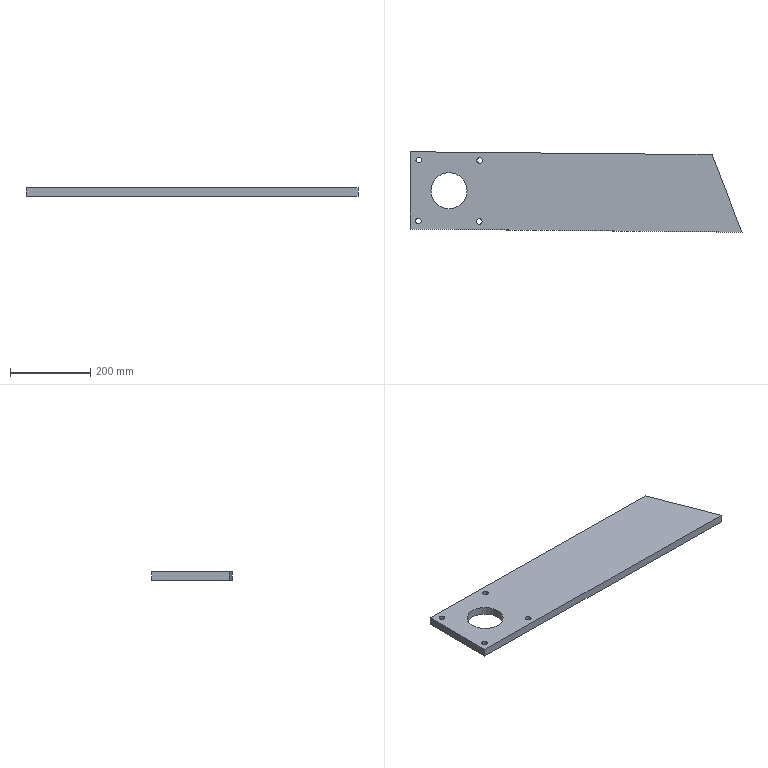Part | SolidWorks | features BaseBody 1 | 1 solid | 16 faces | box 828.827 x 200.894 x 20 mm | volume 2911165 mm3 | cylinder 10 | plane 6 | commonest cylinder face diameters 14.376 x6 14.371 x2 90 x2
STEP:
#1=CARTESIAN_POINT('',(1275.714,2622.106,20.));
#2=VERTEX_POINT('',#1);
#3=CARTESIAN_POINT('',(1290.09,2622.106,20.));
#4=VERTEX_POINT('',#3);
#5=CARTESIAN_POINT('',(1282.902,2622.106,20.));
#6=DIRECTION('',(0.,0.,1.));
#7=DIRECTION('',(1.,0.,0.));
#8=AXIS2_PLACEMENT_3D('',#5,#6,#7);
#9=CIRCLE('',#8,7.188);
#10=EDGE_CURVE('',#2,#4,#9,.T.);
#11=ORIENTED_EDGE('',*,*,#10,.T.);
#12=CARTESIAN_POINT('',(1290.09,2622.106,0.));
#13=VERTEX_POINT('',#12);
#14=CARTESIAN_POINT('',(1290.09,2622.106,20.));
#15=DIRECTION('',(0.,0.,-1.));
#16=VECTOR('',#15,1000.);
#17=LINE('',#14,#16);
#18=EDGE_CURVE('',#4,#13,#17,.T.);
#19=ORIENTED_EDGE('',*,*,#18,.T.);
#20=CARTESIAN_POINT('',(1275.714,2622.106,0.));
#21=VERTEX_POINT('',#20);
#22=CARTESIAN_POINT('',(1282.902,2622.106,0.));
#23=DIRECTION('',(0.,0.,1.));
#24=DIRECTION('',(1.,0.,0.));
#25=AXIS2_PLACEMENT_3D('',#22,#23,#24);
#26=CIRCLE('',#25,7.188);
#27=EDGE_CURVE('',#21,#13,#26,.T.);
#28=ORIENTED_EDGE('',*,*,#27,.F.);
#29=CARTESIAN_POINT('',(1275.714,2622.106,20.));
#30=DIRECTION('',(0.,0.,-1.));
#31=VECTOR('',#30,1000.);
#32=LINE('',#29,#31);
#33=EDGE_CURVE('',#2,#21,#32,.T.);
#34=ORIENTED_EDGE('',*,*,#33,.F.);
#35=EDGE_LOOP('',(#11,#19,#28,#34));
#36=FACE_OUTER_BOUND('',#35,.T.);
#37=CARTESIAN_POINT('',(1282.902,2622.106,20.));
#38=DIRECTION('',(0.,0.,-1.));
#39=DIRECTION('',(-1.,0.,0.));
#40=AXIS2_PLACEMENT_3D('',#37,#38,#39);
#41=CYLINDRICAL_SURFACE('',#40,7.188);
#42=ADVANCED_FACE('',(#36),#41,.F.);
#43=CARTESIAN_POINT('',(1427.707,2620.657,20.));
#44=VERTEX_POINT('',#43);
#45=CARTESIAN_POINT('',(1442.083,2620.657,20.));
#46=VERTEX_POINT('',#45);
#47=CARTESIAN_POINT('',(1434.895,2620.657,20.));
#48=DIRECTION('',(0.,0.,1.));
#49=DIRECTION('',(1.,0.,0.));
#50=AXIS2_PLACEMENT_3D('',#47,#48,#49);
#51=CIRCLE('',#50,7.188);
#52=EDGE_CURVE('',#44,#46,#51,.T.);
#53=ORIENTED_EDGE('',*,*,#52,.T.);
#54=CARTESIAN_POINT('',(1442.083,2620.657,0.));
#55=VERTEX_POINT('',#54);
#56=CARTESIAN_POINT('',(1442.083,2620.657,20.));
#57=DIRECTION('',(0.,0.,-1.));
#58=VECTOR('',#57,1000.);
#59=LINE('',#56,#58);
#60=EDGE_CURVE('',#46,#55,#59,.T.);
#61=ORIENTED_EDGE('',*,*,#60,.T.);
#62=CARTESIAN_POINT('',(1427.707,2620.657,0.));
#63=VERTEX_POINT('',#62);
#64=CARTESIAN_POINT('',(1434.895,2620.657,0.));
#65=DIRECTION('',(0.,0.,1.));
#66=DIRECTION('',(1.,0.,0.));
#67=AXIS2_PLACEMENT_3D('',#64,#65,#66);
#68=CIRCLE('',#67,7.188);
#69=EDGE_CURVE('',#63,#55,#68,.T.);
#70=ORIENTED_EDGE('',*,*,#69,.F.);
#71=CARTESIAN_POINT('',(1427.707,2620.657,20.));
#72=DIRECTION('',(0.,0.,-1.));
#73=VECTOR('',#72,1000.);
#74=LINE('',#71,#73);
#75=EDGE_CURVE('',#44,#63,#74,.T.);
#76=ORIENTED_EDGE('',*,*,#75,.F.);
#77=EDGE_LOOP('',(#53,#61,#70,#76));
#78=FACE_OUTER_BOUND('',#77,.T.);
#79=CARTESIAN_POINT('',(1434.895,2620.657,20.));
#80=DIRECTION('',(0.,0.,-1.));
#81=DIRECTION('',(-1.,0.,0.));
#82=AXIS2_PLACEMENT_3D('',#79,#80,#81);
#83=CYLINDRICAL_SURFACE('',#82,7.188);
#84=ADVANCED_FACE('',(#78),#83,.F.);
#85=CARTESIAN_POINT('',(1429.156,2772.65,20.));
#86=VERTEX_POINT('',#85);
#87=CARTESIAN_POINT('',(1443.533,2772.65,20.));
#88=VERTEX_POINT('',#87);
#89=CARTESIAN_POINT('',(1436.345,2772.65,20.));
#90=DIRECTION('',(0.,0.,1.));
#91=DIRECTION('',(1.,0.,0.));
#92=AXIS2_PLACEMENT_3D('',#89,#90,#91);
#93=CIRCLE('',#92,7.188);
#94=EDGE_CURVE('',#86,#88,#93,.T.);
#95=ORIENTED_EDGE('',*,*,#94,.T.);
#96=CARTESIAN_POINT('',(1443.533,2772.65,0.));
#97=VERTEX_POINT('',#96);
#98=CARTESIAN_POINT('',(1443.533,2772.65,20.));
#99=DIRECTION('',(0.,0.,-1.));
#100=VECTOR('',#99,1000.);
#101=LINE('',#98,#100);
#102=EDGE_CURVE('',#88,#97,#101,.T.);
#103=ORIENTED_EDGE('',*,*,#102,.T.);
#104=CARTESIAN_POINT('',(1429.156,2772.65,0.));
#105=VERTEX_POINT('',#104);
#106=CARTESIAN_POINT('',(1436.345,2772.65,0.));
#107=DIRECTION('',(0.,0.,1.));
#108=DIRECTION('',(1.,0.,0.));
#109=AXIS2_PLACEMENT_3D('',#106,#107,#108);
#110=CIRCLE('',#109,7.188);
#111=EDGE_CURVE('',#105,#97,#110,.T.);
#112=ORIENTED_EDGE('',*,*,#111,.F.);
#113=CARTESIAN_POINT('',(1429.156,2772.65,20.));
#114=DIRECTION('',(0.,0.,-1.));
#115=VECTOR('',#114,1000.);
#116=LINE('',#113,#115);
#117=EDGE_CURVE('',#86,#105,#116,.T.);
#118=ORIENTED_EDGE('',*,*,#117,.F.);
#119=EDGE_LOOP('',(#95,#103,#112,#118));
#120=FACE_OUTER_BOUND('',#119,.T.);
#121=CARTESIAN_POINT('',(1436.345,2772.65,20.));
#122=DIRECTION('',(0.,0.,-1.));
#123=DIRECTION('',(-1.,0.,0.));
#124=AXIS2_PLACEMENT_3D('',#121,#122,#123);
#125=CYLINDRICAL_SURFACE('',#124,7.188);
#126=ADVANCED_FACE('',(#120),#125,.F.);
#127=CARTESIAN_POINT('',(1277.166,2774.099,20.));
#128=VERTEX_POINT('',#127);
#129=CARTESIAN_POINT('',(1291.537,2774.099,20.));
#130=VERTEX_POINT('',#129);
#131=CARTESIAN_POINT('',(1284.351,2774.099,20.));
#132=DIRECTION('',(0.,0.,1.));
#133=DIRECTION('',(1.,0.,0.));
#134=AXIS2_PLACEMENT_3D('',#131,#132,#133);
#135=CIRCLE('',#134,7.186);
#136=EDGE_CURVE('',#128,#130,#135,.T.);
#137=ORIENTED_EDGE('',*,*,#136,.T.);
#138=CARTESIAN_POINT('',(1291.537,2774.099,0.));
#139=VERTEX_POINT('',#138);
#140=CARTESIAN_POINT('',(1291.537,2774.099,20.));
#141=DIRECTION('',(0.,0.,-1.));
#142=VECTOR('',#141,1000.);
#143=LINE('',#140,#142);
#144=EDGE_CURVE('',#130,#139,#143,.T.);
#145=ORIENTED_EDGE('',*,*,#144,.T.);
#146=CARTESIAN_POINT('',(1277.166,2774.099,0.));
#147=VERTEX_POINT('',#146);
#148=CARTESIAN_POINT('',(1284.351,2774.099,0.));
#149=DIRECTION('',(0.,0.,1.));
#150=DIRECTION('',(1.,0.,0.));
#151=AXIS2_PLACEMENT_3D('',#148,#149,#150);
#152=CIRCLE('',#151,7.186);
#153=EDGE_CURVE('',#147,#139,#152,.T.);
#154=ORIENTED_EDGE('',*,*,#153,.F.);
#155=CARTESIAN_POINT('',(1277.166,2774.099,20.));
#156=DIRECTION('',(0.,0.,-1.));
#157=VECTOR('',#156,1000.);
#158=LINE('',#155,#157);
#159=EDGE_CURVE('',#128,#147,#158,.T.);
#160=ORIENTED_EDGE('',*,*,#159,.F.);
#161=EDGE_LOOP('',(#137,#145,#154,#160));
#162=FACE_OUTER_BOUND('',#161,.T.);
#163=CARTESIAN_POINT('',(1284.351,2774.099,20.));
#164=DIRECTION('',(0.,0.,-1.));
#165=DIRECTION('',(-1.,0.,0.));
#166=AXIS2_PLACEMENT_3D('',#163,#164,#165);
#167=CYLINDRICAL_SURFACE('',#166,7.186);
#168=ADVANCED_FACE('',(#162),#167,.F.);
#169=CARTESIAN_POINT('',(1314.623,2697.378,20.));
#170=VERTEX_POINT('',#169);
#171=CARTESIAN_POINT('',(1404.623,2697.378,20.));
#172=VERTEX_POINT('',#171);
#173=CARTESIAN_POINT('',(1359.623,2697.378,20.));
#174=DIRECTION('',(0.,0.,1.));
#175=DIRECTION('',(1.,0.,0.));
#176=AXIS2_PLACEMENT_3D('',#173,#174,#175);
#177=CIRCLE('',#176,45.);
#178=EDGE_CURVE('',#170,#172,#177,.T.);
#179=ORIENTED_EDGE('',*,*,#178,.T.);
#180=CARTESIAN_POINT('',(1404.623,2697.378,0.));
#181=VERTEX_POINT('',#180);
#182=CARTESIAN_POINT('',(1404.623,2697.378,20.));
#183=DIRECTION('',(0.,0.,-1.));
#184=VECTOR('',#183,1000.);
#185=LINE('',#182,#184);
#186=EDGE_CURVE('',#172,#181,#185,.T.);
#187=ORIENTED_EDGE('',*,*,#186,.T.);
#188=CARTESIAN_POINT('',(1314.623,2697.378,0.));
#189=VERTEX_POINT('',#188);
#190=CARTESIAN_POINT('',(1359.623,2697.378,0.));
#191=DIRECTION('',(0.,0.,1.));
#192=DIRECTION('',(1.,0.,0.));
#193=AXIS2_PLACEMENT_3D('',#190,#191,#192);
#194=CIRCLE('',#193,45.);
#195=EDGE_CURVE('',#189,#181,#194,.T.);
#196=ORIENTED_EDGE('',*,*,#195,.F.);
#197=CARTESIAN_POINT('',(1314.623,2697.378,20.));
#198=DIRECTION('',(0.,0.,-1.));
#199=VECTOR('',#198,1000.);
#200=LINE('',#197,#199);
#201=EDGE_CURVE('',#170,#189,#200,.T.);
#202=ORIENTED_EDGE('',*,*,#201,.F.);
#203=EDGE_LOOP('',(#179,#187,#196,#202));
#204=FACE_OUTER_BOUND('',#203,.T.);
#205=CARTESIAN_POINT('',(1359.623,2697.378,20.));
#206=DIRECTION('',(0.,0.,-1.));
#207=DIRECTION('',(-1.,0.,0.));
#208=AXIS2_PLACEMENT_3D('',#205,#206,#207);
#209=CYLINDRICAL_SURFACE('',#208,45.);
#210=ADVANCED_FACE('',(#204),#209,.F.);
#211=ORIENTED_EDGE('',*,*,#52,.F.);
#212=CARTESIAN_POINT('',(1434.895,2620.657,20.));
#213=DIRECTION('',(0.,0.,1.));
#214=DIRECTION('',(1.,0.,0.));
#215=AXIS2_PLACEMENT_3D('',#212,#213,#214);
#216=CIRCLE('',#215,7.188);
#217=EDGE_CURVE('',#46,#44,#216,.T.);
#218=ORIENTED_EDGE('',*,*,#217,.F.);
#219=EDGE_LOOP('',(#211,#218));
#220=FACE_BOUND('',#219,.T.);
#221=ORIENTED_EDGE('',*,*,#136,.F.);
#222=CARTESIAN_POINT('',(1284.351,2774.099,20.));
#223=DIRECTION('',(0.,0.,1.));
#224=DIRECTION('',(1.,0.,0.));
#225=AXIS2_PLACEMENT_3D('',#222,#223,#224);
#226=CIRCLE('',#225,7.186);
#227=EDGE_CURVE('',#130,#128,#226,.T.);
#228=ORIENTED_EDGE('',*,*,#227,.F.);
#229=EDGE_LOOP('',(#221,#228));
#230=FACE_BOUND('',#229,.T.);
#231=CARTESIAN_POINT('',(1264.048,2794.794,20.));
#232=VERTEX_POINT('',#231);
#233=CARTESIAN_POINT('',(1262.208,2601.803,20.));
#234=VERTEX_POINT('',#233);
#235=CARTESIAN_POINT('',(1264.048,2794.794,20.));
#236=DIRECTION('',(-0.009534,-1.,0.));
#237=VECTOR('',#236,1000.);
#238=LINE('',#235,#237);
#239=EDGE_CURVE('',#232,#234,#238,.T.);
#240=ORIENTED_EDGE('',*,*,#239,.T.);
#241=CARTESIAN_POINT('',(2091.035,2593.9,20.));
#242=VERTEX_POINT('',#241);
#243=CARTESIAN_POINT('',(1262.208,2601.803,20.));
#244=DIRECTION('',(1.,-0.009534,0.));
#245=VECTOR('',#244,1000.);
#246=LINE('',#243,#245);
#247=EDGE_CURVE('',#234,#242,#246,.T.);
#248=ORIENTED_EDGE('',*,*,#247,.T.);
#249=CARTESIAN_POINT('',(2016.176,2787.622,20.));
#250=VERTEX_POINT('',#249);
#251=CARTESIAN_POINT('',(2019.781,2778.295,20.));
#252=DIRECTION('',(-0.3604,0.9328,0.));
#253=VECTOR('',#252,1000.);
#254=LINE('',#251,#253);
#255=EDGE_CURVE('',#242,#250,#254,.T.);
#256=ORIENTED_EDGE('',*,*,#255,.T.);
#257=CARTESIAN_POINT('',(1264.048,2794.794,20.));
#258=DIRECTION('',(-1.,0.009534,0.));
#259=VECTOR('',#258,1000.);
#260=LINE('',#257,#259);
#261=EDGE_CURVE('',#250,#232,#260,.T.);
#262=ORIENTED_EDGE('',*,*,#261,.T.);
#263=EDGE_LOOP('',(#240,#248,#256,#262));
#264=FACE_OUTER_BOUND('',#263,.T.);
#265=ORIENTED_EDGE('',*,*,#178,.F.);
#266=CARTESIAN_POINT('',(1359.623,2697.378,20.));
#267=DIRECTION('',(0.,0.,1.));
#268=DIRECTION('',(1.,0.,0.));
#269=AXIS2_PLACEMENT_3D('',#266,#267,#268);
#270=CIRCLE('',#269,45.);
#271=EDGE_CURVE('',#172,#170,#270,.T.);
#272=ORIENTED_EDGE('',*,*,#271,.F.);
#273=EDGE_LOOP('',(#265,#272));
#274=FACE_BOUND('',#273,.T.);
#275=ORIENTED_EDGE('',*,*,#94,.F.);
#276=CARTESIAN_POINT('',(1436.345,2772.65,20.));
#277=DIRECTION('',(0.,0.,1.));
#278=DIRECTION('',(1.,0.,0.));
#279=AXIS2_PLACEMENT_3D('',#276,#277,#278);
#280=CIRCLE('',#279,7.188);
#281=EDGE_CURVE('',#88,#86,#280,.T.);
#282=ORIENTED_EDGE('',*,*,#281,.F.);
#283=EDGE_LOOP('',(#275,#282));
#284=FACE_BOUND('',#283,.T.);
#285=ORIENTED_EDGE('',*,*,#10,.F.);
#286=CARTESIAN_POINT('',(1282.902,2622.106,20.));
#287=DIRECTION('',(0.,0.,1.));
#288=DIRECTION('',(1.,0.,0.));
#289=AXIS2_PLACEMENT_3D('',#286,#287,#288);
#290=CIRCLE('',#289,7.188);
#291=EDGE_CURVE('',#4,#2,#290,.T.);
#292=ORIENTED_EDGE('',*,*,#291,.F.);
#293=EDGE_LOOP('',(#285,#292));
#294=FACE_BOUND('',#293,.T.);
#295=CARTESIAN_POINT('',(0.,0.,20.));
#296=DIRECTION('',(0.,0.,1.));
#297=DIRECTION('',(1.,0.,0.));
#298=AXIS2_PLACEMENT_3D('',#295,#296,#297);
#299=PLANE('',#298);
#300=ADVANCED_FACE('',(#220,#230,#264,#274,#284,#294),#299,.T.);
#301=CARTESIAN_POINT('',(1264.048,2794.794,0.));
#302=VERTEX_POINT('',#301);
#303=CARTESIAN_POINT('',(1262.208,2601.803,0.));
#304=VERTEX_POINT('',#303);
#305=CARTESIAN_POINT('',(1264.048,2794.794,0.));
#306=DIRECTION('',(-0.009534,-1.,0.));
#307=VECTOR('',#306,1000.);
#308=LINE('',#305,#307);
#309=EDGE_CURVE('',#302,#304,#308,.T.);
#310=ORIENTED_EDGE('',*,*,#309,.F.);
#311=CARTESIAN_POINT('',(2016.176,2787.622,0.));
#312=VERTEX_POINT('',#311);
#313=CARTESIAN_POINT('',(1264.048,2794.794,0.));
#314=DIRECTION('',(-1.,0.009534,0.));
#315=VECTOR('',#314,1000.);
#316=LINE('',#313,#315);
#317=EDGE_CURVE('',#312,#302,#316,.T.);
#318=ORIENTED_EDGE('',*,*,#317,.F.);
#319=CARTESIAN_POINT('',(2091.035,2593.9,0.));
#320=VERTEX_POINT('',#319);
#321=CARTESIAN_POINT('',(2019.781,2778.295,0.));
#322=DIRECTION('',(-0.3604,0.9328,0.));
#323=VECTOR('',#322,1000.);
#324=LINE('',#321,#323);
#325=EDGE_CURVE('',#320,#312,#324,.T.);
#326=ORIENTED_EDGE('',*,*,#325,.F.);
#327=CARTESIAN_POINT('',(1262.208,2601.803,0.));
#328=DIRECTION('',(1.,-0.009534,0.));
#329=VECTOR('',#328,1000.);
#330=LINE('',#327,#329);
#331=EDGE_CURVE('',#304,#320,#330,.T.);
#332=ORIENTED_EDGE('',*,*,#331,.F.);
#333=EDGE_LOOP('',(#310,#318,#326,#332));
#334=FACE_OUTER_BOUND('',#333,.T.);
#335=ORIENTED_EDGE('',*,*,#195,.T.);
#336=CARTESIAN_POINT('',(1359.623,2697.378,0.));
#337=DIRECTION('',(0.,0.,1.));
#338=DIRECTION('',(1.,0.,0.));
#339=AXIS2_PLACEMENT_3D('',#336,#337,#338);
#340=CIRCLE('',#339,45.);
#341=EDGE_CURVE('',#181,#189,#340,.T.);
#342=ORIENTED_EDGE('',*,*,#341,.T.);
#343=EDGE_LOOP('',(#335,#342));
#344=FACE_BOUND('',#343,.T.);
#345=ORIENTED_EDGE('',*,*,#153,.T.);
#346=CARTESIAN_POINT('',(1284.351,2774.099,0.));
#347=DIRECTION('',(0.,0.,1.));
#348=DIRECTION('',(1.,0.,0.));
#349=AXIS2_PLACEMENT_3D('',#346,#347,#348);
#350=CIRCLE('',#349,7.186);
#351=EDGE_CURVE('',#139,#147,#350,.T.);
#352=ORIENTED_EDGE('',*,*,#351,.T.);
#353=EDGE_LOOP('',(#345,#352));
#354=FACE_BOUND('',#353,.T.);
#355=ORIENTED_EDGE('',*,*,#111,.T.);
#356=CARTESIAN_POINT('',(1436.345,2772.65,0.));
#357=DIRECTION('',(0.,0.,1.));
#358=DIRECTION('',(1.,0.,0.));
#359=AXIS2_PLACEMENT_3D('',#356,#357,#358);
#360=CIRCLE('',#359,7.188);
#361=EDGE_CURVE('',#97,#105,#360,.T.);
#362=ORIENTED_EDGE('',*,*,#361,.T.);
#363=EDGE_LOOP('',(#355,#362));
#364=FACE_BOUND('',#363,.T.);
#365=ORIENTED_EDGE('',*,*,#69,.T.);
#366=CARTESIAN_POINT('',(1434.895,2620.657,0.));
#367=DIRECTION('',(0.,0.,1.));
#368=DIRECTION('',(1.,0.,0.));
#369=AXIS2_PLACEMENT_3D('',#366,#367,#368);
#370=CIRCLE('',#369,7.188);
#371=EDGE_CURVE('',#55,#63,#370,.T.);
#372=ORIENTED_EDGE('',*,*,#371,.T.);
#373=EDGE_LOOP('',(#365,#372));
#374=FACE_BOUND('',#373,.T.);
#375=ORIENTED_EDGE('',*,*,#27,.T.);
#376=CARTESIAN_POINT('',(1282.902,2622.106,0.));
#377=DIRECTION('',(0.,0.,1.));
#378=DIRECTION('',(1.,0.,0.));
#379=AXIS2_PLACEMENT_3D('',#376,#377,#378);
#380=CIRCLE('',#379,7.188);
#381=EDGE_CURVE('',#13,#21,#380,.T.);
#382=ORIENTED_EDGE('',*,*,#381,.T.);
#383=EDGE_LOOP('',(#375,#382));
#384=FACE_BOUND('',#383,.T.);
#385=CARTESIAN_POINT('',(0.,0.,0.));
#386=DIRECTION('',(0.,0.,1.));
#387=DIRECTION('',(1.,0.,0.));
#388=AXIS2_PLACEMENT_3D('',#385,#386,#387);
#389=PLANE('',#388);
#390=ADVANCED_FACE('',(#334,#344,#354,#364,#374,#384),#389,.F.);
#391=ORIENTED_EDGE('',*,*,#309,.T.);
#392=CARTESIAN_POINT('',(1262.208,2601.803,20.));
#393=DIRECTION('',(0.,0.,-1.));
#394=VECTOR('',#393,1000.);
#395=LINE('',#392,#394);
#396=EDGE_CURVE('',#234,#304,#395,.T.);
#397=ORIENTED_EDGE('',*,*,#396,.F.);
#398=ORIENTED_EDGE('',*,*,#239,.F.);
#399=CARTESIAN_POINT('',(1264.048,2794.794,20.));
#400=DIRECTION('',(0.,0.,-1.));
#401=VECTOR('',#400,1000.);
#402=LINE('',#399,#401);
#403=EDGE_CURVE('',#232,#302,#402,.T.);
#404=ORIENTED_EDGE('',*,*,#403,.T.);
#405=EDGE_LOOP('',(#391,#397,#398,#404));
#406=FACE_OUTER_BOUND('',#405,.T.);
#407=CARTESIAN_POINT('',(1264.048,2794.794,20.));
#408=DIRECTION('',(1.,-0.009534,0.));
#409=DIRECTION('',(0.009534,1.,0.));
#410=AXIS2_PLACEMENT_3D('',#407,#408,#409);
#411=PLANE('',#410);
#412=ADVANCED_FACE('',(#406),#411,.F.);
#413=ORIENTED_EDGE('',*,*,#331,.T.);
#414=CARTESIAN_POINT('',(2091.035,2593.9,20.));
#415=DIRECTION('',(0.,0.,-1.));
#416=VECTOR('',#415,1000.);
#417=LINE('',#414,#416);
#418=EDGE_CURVE('',#242,#320,#417,.T.);
#419=ORIENTED_EDGE('',*,*,#418,.F.);
#420=ORIENTED_EDGE('',*,*,#247,.F.);
#421=ORIENTED_EDGE('',*,*,#396,.T.);
#422=EDGE_LOOP('',(#413,#419,#420,#421));
#423=FACE_OUTER_BOUND('',#422,.T.);
#424=CARTESIAN_POINT('',(1262.208,2601.803,20.));
#425=DIRECTION('',(0.009534,1.,0.));
#426=DIRECTION('',(-1.,0.009534,0.));
#427=AXIS2_PLACEMENT_3D('',#424,#425,#426);
#428=PLANE('',#427);
#429=ADVANCED_FACE('',(#423),#428,.F.);
#430=ORIENTED_EDGE('',*,*,#325,.T.);
#431=CARTESIAN_POINT('',(2016.176,2787.622,20.));
#432=DIRECTION('',(0.,0.,-1.));
#433=VECTOR('',#432,1000.);
#434=LINE('',#431,#433);
#435=EDGE_CURVE('',#250,#312,#434,.T.);
#436=ORIENTED_EDGE('',*,*,#435,.F.);
#437=ORIENTED_EDGE('',*,*,#255,.F.);
#438=ORIENTED_EDGE('',*,*,#418,.T.);
#439=EDGE_LOOP('',(#430,#436,#437,#438));
#440=FACE_OUTER_BOUND('',#439,.T.);
#441=CARTESIAN_POINT('',(2019.781,2778.295,20.));
#442=DIRECTION('',(-0.9328,-0.3604,0.));
#443=DIRECTION('',(0.3604,-0.9328,0.));
#444=AXIS2_PLACEMENT_3D('',#441,#442,#443);
#445=PLANE('',#444);
#446=ADVANCED_FACE('',(#440),#445,.F.);
#447=ORIENTED_EDGE('',*,*,#317,.T.);
#448=ORIENTED_EDGE('',*,*,#403,.F.);
#449=ORIENTED_EDGE('',*,*,#261,.F.);
#450=ORIENTED_EDGE('',*,*,#435,.T.);
#451=EDGE_LOOP('',(#447,#448,#449,#450));
#452=FACE_OUTER_BOUND('',#451,.T.);
#453=CARTESIAN_POINT('',(1264.048,2794.794,20.));
#454=DIRECTION('',(-0.009534,-1.,0.));
#455=DIRECTION('',(1.,-0.009534,0.));
#456=AXIS2_PLACEMENT_3D('',#453,#454,#455);
#457=PLANE('',#456);
#458=ADVANCED_FACE('',(#452),#457,.F.);
#459=ORIENTED_EDGE('',*,*,#186,.F.);
#460=ORIENTED_EDGE('',*,*,#271,.T.);
#461=ORIENTED_EDGE('',*,*,#201,.T.);
#462=ORIENTED_EDGE('',*,*,#341,.F.);
#463=EDGE_LOOP('',(#459,#460,#461,#462));
#464=FACE_OUTER_BOUND('',#463,.T.);
#465=CARTESIAN_POINT('',(1359.623,2697.378,20.));
#466=DIRECTION('',(0.,0.,-1.));
#467=DIRECTION('',(-1.,0.,0.));
#468=AXIS2_PLACEMENT_3D('',#465,#466,#467);
#469=CYLINDRICAL_SURFACE('',#468,45.);
#470=ADVANCED_FACE('',(#464),#469,.F.);
#471=ORIENTED_EDGE('',*,*,#144,.F.);
#472=ORIENTED_EDGE('',*,*,#227,.T.);
#473=ORIENTED_EDGE('',*,*,#159,.T.);
#474=ORIENTED_EDGE('',*,*,#351,.F.);
#475=EDGE_LOOP('',(#471,#472,#473,#474));
#476=FACE_OUTER_BOUND('',#475,.T.);
#477=CARTESIAN_POINT('',(1284.351,2774.099,20.));
#478=DIRECTION('',(0.,0.,-1.));
#479=DIRECTION('',(-1.,0.,0.));
#480=AXIS2_PLACEMENT_3D('',#477,#478,#479);
#481=CYLINDRICAL_SURFACE('',#480,7.186);
#482=ADVANCED_FACE('',(#476),#481,.F.);
#483=ORIENTED_EDGE('',*,*,#102,.F.);
#484=ORIENTED_EDGE('',*,*,#281,.T.);
#485=ORIENTED_EDGE('',*,*,#117,.T.);
#486=ORIENTED_EDGE('',*,*,#361,.F.);
#487=EDGE_LOOP('',(#483,#484,#485,#486));
#488=FACE_OUTER_BOUND('',#487,.T.);
#489=CARTESIAN_POINT('',(1436.345,2772.65,20.));
#490=DIRECTION('',(0.,0.,-1.));
#491=DIRECTION('',(-1.,0.,0.));
#492=AXIS2_PLACEMENT_3D('',#489,#490,#491);
#493=CYLINDRICAL_SURFACE('',#492,7.188);
#494=ADVANCED_FACE('',(#488),#493,.F.);
#495=ORIENTED_EDGE('',*,*,#60,.F.);
#496=ORIENTED_EDGE('',*,*,#217,.T.);
#497=ORIENTED_EDGE('',*,*,#75,.T.);
#498=ORIENTED_EDGE('',*,*,#371,.F.);
#499=EDGE_LOOP('',(#495,#496,#497,#498));
#500=FACE_OUTER_BOUND('',#499,.T.);
#501=CARTESIAN_POINT('',(1434.895,2620.657,20.));
#502=DIRECTION('',(0.,0.,-1.));
#503=DIRECTION('',(-1.,0.,0.));
#504=AXIS2_PLACEMENT_3D('',#501,#502,#503);
#505=CYLINDRICAL_SURFACE('',#504,7.188);
#506=ADVANCED_FACE('',(#500),#505,.F.);
#507=ORIENTED_EDGE('',*,*,#18,.F.);
#508=ORIENTED_EDGE('',*,*,#291,.T.);
#509=ORIENTED_EDGE('',*,*,#33,.T.);
#510=ORIENTED_EDGE('',*,*,#381,.F.);
#511=EDGE_LOOP('',(#507,#508,#509,#510));
#512=FACE_OUTER_BOUND('',#511,.T.);
#513=CARTESIAN_POINT('',(1282.902,2622.106,20.));
#514=DIRECTION('',(0.,0.,-1.));
#515=DIRECTION('',(-1.,0.,0.));
#516=AXIS2_PLACEMENT_3D('',#513,#514,#515);
#517=CYLINDRICAL_SURFACE('',#516,7.188);
#518=ADVANCED_FACE('',(#512),#517,.F.);
#519=CLOSED_SHELL('',(#42,#84,#126,#168,#210,#300,#390,#412,#429,#446,#458,#470,#482,#494,#506,#518));
#520=MANIFOLD_SOLID_BREP('',#519);
#521=CARTESIAN_POINT('',(0.,0.,0.));
#522=DIRECTION('',(0.,0.,1.));
#523=DIRECTION('',(1.,0.,0.));
#524=AXIS2_PLACEMENT_3D('',#521,#522,#523);
#525=(LENGTH_UNIT()NAMED_UNIT(*)SI_UNIT(.MILLI.,.METRE.));
#526=UNCERTAINTY_MEASURE_WITH_UNIT(LENGTH_MEASURE(0.00001),#525,'','');
#527=(NAMED_UNIT(*)PLANE_ANGLE_UNIT()SI_UNIT($,.RADIAN.));
#528=(NAMED_UNIT(*)SI_UNIT($,.STERADIAN.)SOLID_ANGLE_UNIT());
#529=(GEOMETRIC_REPRESENTATION_CONTEXT(3)GLOBAL_UNCERTAINTY_ASSIGNED_CONTEXT((#526))GLOBAL_UNIT_ASSIGNED_CONTEXT((#525,#527,#528))REPRESENTATION_CONTEXT('',''));
#530=ADVANCED_BREP_SHAPE_REPRESENTATION('',(#520,#524),#529);